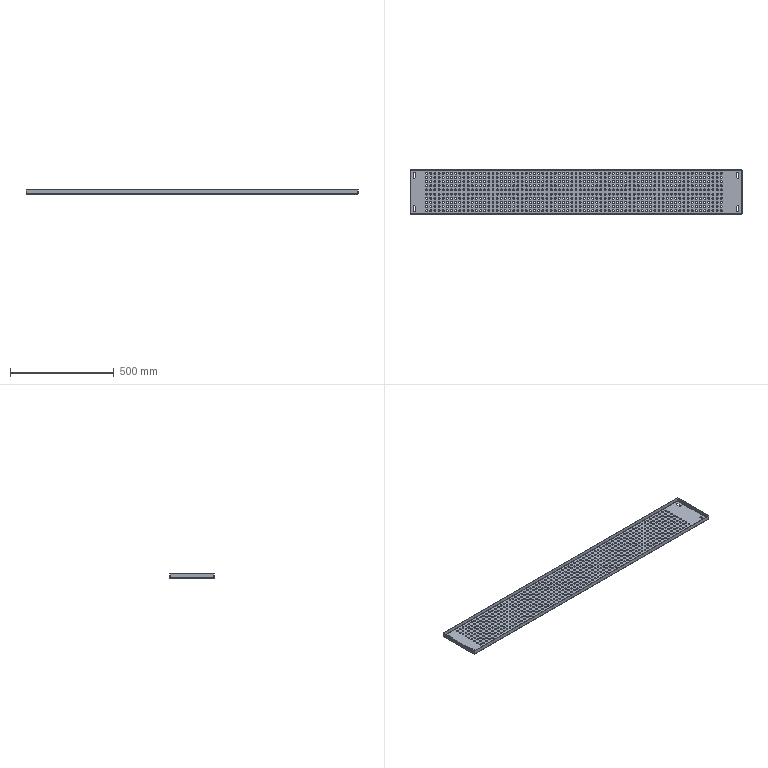Part | SolidWorks | features ICE 3, EdgeFlange 1, Extrusion 1, FlatPattern 1, SheetMetal 1, SolidToSheetMetal 1 | 1 solid | 1494 faces | box 1600 x 215 x 20 mm | volume 538674 mm3 | cylinder 1456 | plane 30 | spline 8 | commonest cylinder face diameters 9.2 x1440 10 x8 2 x4 5 x4